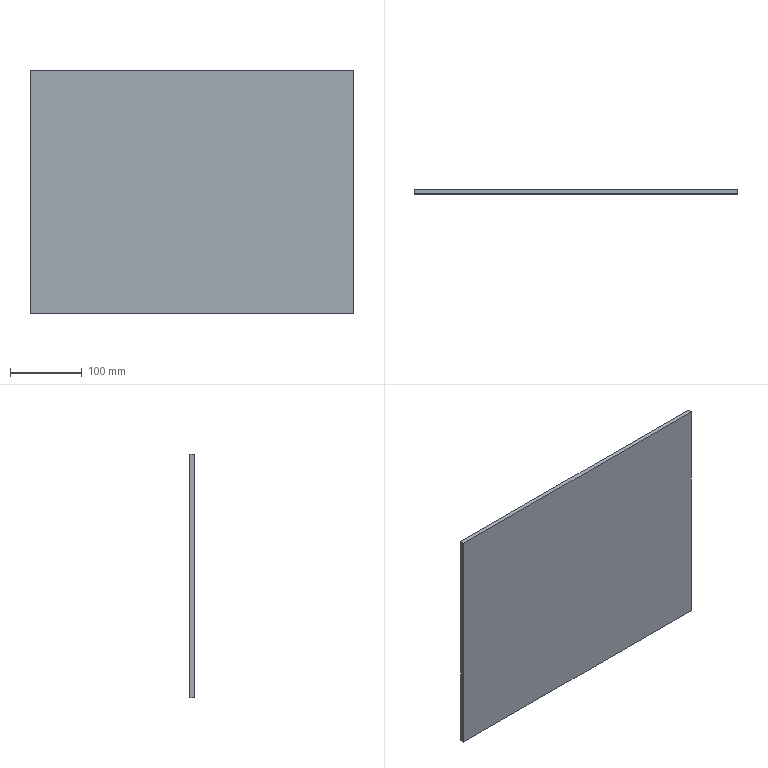Part | SolidWorks | features Extrusion 1 | 1 solid | 6 faces | box 450 x 6 x 340 mm | volume 918000 mm3 | plane 6
STEP:
#1=CARTESIAN_POINT('',(50.,-5.,-400.));
#2=VERTEX_POINT('',#1);
#3=CARTESIAN_POINT('',(50.,-5.,-60.));
#4=VERTEX_POINT('',#3);
#5=CARTESIAN_POINT('',(50.,-5.,-400.));
#6=DIRECTION('',(0.,0.,1.));
#7=VECTOR('',#6,1000.);
#8=LINE('',#5,#7);
#9=EDGE_CURVE('',#2,#4,#8,.T.);
#10=ORIENTED_EDGE('',*,*,#9,.F.);
#11=CARTESIAN_POINT('',(50.,-11.,-400.));
#12=VERTEX_POINT('',#11);
#13=CARTESIAN_POINT('',(50.,-11.,-400.));
#14=DIRECTION('',(0.,1.,0.));
#15=VECTOR('',#14,1000.);
#16=LINE('',#13,#15);
#17=EDGE_CURVE('',#12,#2,#16,.T.);
#18=ORIENTED_EDGE('',*,*,#17,.F.);
#19=CARTESIAN_POINT('',(50.,-11.,-60.));
#20=VERTEX_POINT('',#19);
#21=CARTESIAN_POINT('',(50.,-11.,-400.));
#22=DIRECTION('',(0.,0.,1.));
#23=VECTOR('',#22,1000.);
#24=LINE('',#21,#23);
#25=EDGE_CURVE('',#12,#20,#24,.T.);
#26=ORIENTED_EDGE('',*,*,#25,.T.);
#27=CARTESIAN_POINT('',(50.,-11.,-60.));
#28=DIRECTION('',(0.,1.,0.));
#29=VECTOR('',#28,1000.);
#30=LINE('',#27,#29);
#31=EDGE_CURVE('',#20,#4,#30,.T.);
#32=ORIENTED_EDGE('',*,*,#31,.T.);
#33=EDGE_LOOP('',(#10,#18,#26,#32));
#34=FACE_OUTER_BOUND('',#33,.T.);
#35=CARTESIAN_POINT('',(50.,-11.,-400.));
#36=DIRECTION('',(-1.,0.,0.));
#37=DIRECTION('',(0.,0.,1.));
#38=AXIS2_PLACEMENT_3D('',#35,#36,#37);
#39=PLANE('',#38);
#40=ADVANCED_FACE('',(#34),#39,.T.);
#41=CARTESIAN_POINT('',(500.,-5.,-400.));
#42=VERTEX_POINT('',#41);
#43=CARTESIAN_POINT('',(500.,-5.,-400.));
#44=DIRECTION('',(-1.,0.,0.));
#45=VECTOR('',#44,1000.);
#46=LINE('',#43,#45);
#47=EDGE_CURVE('',#42,#2,#46,.T.);
#48=ORIENTED_EDGE('',*,*,#47,.F.);
#49=CARTESIAN_POINT('',(500.,-11.,-400.));
#50=VERTEX_POINT('',#49);
#51=CARTESIAN_POINT('',(500.,-11.,-400.));
#52=DIRECTION('',(0.,1.,0.));
#53=VECTOR('',#52,1000.);
#54=LINE('',#51,#53);
#55=EDGE_CURVE('',#50,#42,#54,.T.);
#56=ORIENTED_EDGE('',*,*,#55,.F.);
#57=CARTESIAN_POINT('',(500.,-11.,-400.));
#58=DIRECTION('',(-1.,0.,0.));
#59=VECTOR('',#58,1000.);
#60=LINE('',#57,#59);
#61=EDGE_CURVE('',#50,#12,#60,.T.);
#62=ORIENTED_EDGE('',*,*,#61,.T.);
#63=ORIENTED_EDGE('',*,*,#17,.T.);
#64=EDGE_LOOP('',(#48,#56,#62,#63));
#65=FACE_OUTER_BOUND('',#64,.T.);
#66=CARTESIAN_POINT('',(500.,-11.,-400.));
#67=DIRECTION('',(0.,0.,-1.));
#68=DIRECTION('',(-1.,0.,0.));
#69=AXIS2_PLACEMENT_3D('',#66,#67,#68);
#70=PLANE('',#69);
#71=ADVANCED_FACE('',(#65),#70,.T.);
#72=CARTESIAN_POINT('',(500.,-5.,-60.));
#73=VERTEX_POINT('',#72);
#74=CARTESIAN_POINT('',(500.,-5.,-60.));
#75=DIRECTION('',(0.,0.,-1.));
#76=VECTOR('',#75,1000.);
#77=LINE('',#74,#76);
#78=EDGE_CURVE('',#73,#42,#77,.T.);
#79=ORIENTED_EDGE('',*,*,#78,.F.);
#80=CARTESIAN_POINT('',(500.,-11.,-60.));
#81=VERTEX_POINT('',#80);
#82=CARTESIAN_POINT('',(500.,-11.,-60.));
#83=DIRECTION('',(0.,1.,0.));
#84=VECTOR('',#83,1000.);
#85=LINE('',#82,#84);
#86=EDGE_CURVE('',#81,#73,#85,.T.);
#87=ORIENTED_EDGE('',*,*,#86,.F.);
#88=CARTESIAN_POINT('',(500.,-11.,-60.));
#89=DIRECTION('',(0.,0.,-1.));
#90=VECTOR('',#89,1000.);
#91=LINE('',#88,#90);
#92=EDGE_CURVE('',#81,#50,#91,.T.);
#93=ORIENTED_EDGE('',*,*,#92,.T.);
#94=ORIENTED_EDGE('',*,*,#55,.T.);
#95=EDGE_LOOP('',(#79,#87,#93,#94));
#96=FACE_OUTER_BOUND('',#95,.T.);
#97=CARTESIAN_POINT('',(500.,-11.,-60.));
#98=DIRECTION('',(1.,0.,0.));
#99=DIRECTION('',(0.,0.,-1.));
#100=AXIS2_PLACEMENT_3D('',#97,#98,#99);
#101=PLANE('',#100);
#102=ADVANCED_FACE('',(#96),#101,.T.);
#103=CARTESIAN_POINT('',(50.,-5.,-60.));
#104=DIRECTION('',(1.,0.,0.));
#105=VECTOR('',#104,1000.);
#106=LINE('',#103,#105);
#107=EDGE_CURVE('',#4,#73,#106,.T.);
#108=ORIENTED_EDGE('',*,*,#107,.F.);
#109=ORIENTED_EDGE('',*,*,#31,.F.);
#110=CARTESIAN_POINT('',(50.,-11.,-60.));
#111=DIRECTION('',(1.,0.,0.));
#112=VECTOR('',#111,1000.);
#113=LINE('',#110,#112);
#114=EDGE_CURVE('',#20,#81,#113,.T.);
#115=ORIENTED_EDGE('',*,*,#114,.T.);
#116=ORIENTED_EDGE('',*,*,#86,.T.);
#117=EDGE_LOOP('',(#108,#109,#115,#116));
#118=FACE_OUTER_BOUND('',#117,.T.);
#119=CARTESIAN_POINT('',(50.,-11.,-60.));
#120=DIRECTION('',(0.,0.,1.));
#121=DIRECTION('',(1.,0.,0.));
#122=AXIS2_PLACEMENT_3D('',#119,#120,#121);
#123=PLANE('',#122);
#124=ADVANCED_FACE('',(#118),#123,.T.);
#125=ORIENTED_EDGE('',*,*,#25,.F.);
#126=ORIENTED_EDGE('',*,*,#61,.F.);
#127=ORIENTED_EDGE('',*,*,#92,.F.);
#128=ORIENTED_EDGE('',*,*,#114,.F.);
#129=EDGE_LOOP('',(#125,#126,#127,#128));
#130=FACE_OUTER_BOUND('',#129,.T.);
#131=CARTESIAN_POINT('',(0.,-11.,0.));
#132=DIRECTION('',(0.,1.,0.));
#133=DIRECTION('',(0.,0.,1.));
#134=AXIS2_PLACEMENT_3D('',#131,#132,#133);
#135=PLANE('',#134);
#136=ADVANCED_FACE('',(#130),#135,.F.);
#137=ORIENTED_EDGE('',*,*,#9,.T.);
#138=ORIENTED_EDGE('',*,*,#107,.T.);
#139=ORIENTED_EDGE('',*,*,#78,.T.);
#140=ORIENTED_EDGE('',*,*,#47,.T.);
#141=EDGE_LOOP('',(#137,#138,#139,#140));
#142=FACE_OUTER_BOUND('',#141,.T.);
#143=CARTESIAN_POINT('',(0.,-5.,0.));
#144=DIRECTION('',(0.,1.,0.));
#145=DIRECTION('',(0.,0.,1.));
#146=AXIS2_PLACEMENT_3D('',#143,#144,#145);
#147=PLANE('',#146);
#148=ADVANCED_FACE('',(#142),#147,.T.);
#149=CLOSED_SHELL('',(#40,#71,#102,#124,#136,#148));
#150=MANIFOLD_SOLID_BREP('',#149);
#151=CARTESIAN_POINT('',(0.,0.,0.));
#152=DIRECTION('',(0.,0.,1.));
#153=DIRECTION('',(1.,0.,0.));
#154=AXIS2_PLACEMENT_3D('',#151,#152,#153);
#155=(LENGTH_UNIT()NAMED_UNIT(*)SI_UNIT(.MILLI.,.METRE.));
#156=UNCERTAINTY_MEASURE_WITH_UNIT(LENGTH_MEASURE(0.00001),#155,'','');
#157=(NAMED_UNIT(*)PLANE_ANGLE_UNIT()SI_UNIT($,.RADIAN.));
#158=(NAMED_UNIT(*)SI_UNIT($,.STERADIAN.)SOLID_ANGLE_UNIT());
#159=(GEOMETRIC_REPRESENTATION_CONTEXT(3)GLOBAL_UNCERTAINTY_ASSIGNED_CONTEXT((#156))GLOBAL_UNIT_ASSIGNED_CONTEXT((#155,#157,#158))REPRESENTATION_CONTEXT('',''));
#160=ADVANCED_BREP_SHAPE_REPRESENTATION('',(#150,#154),#159);